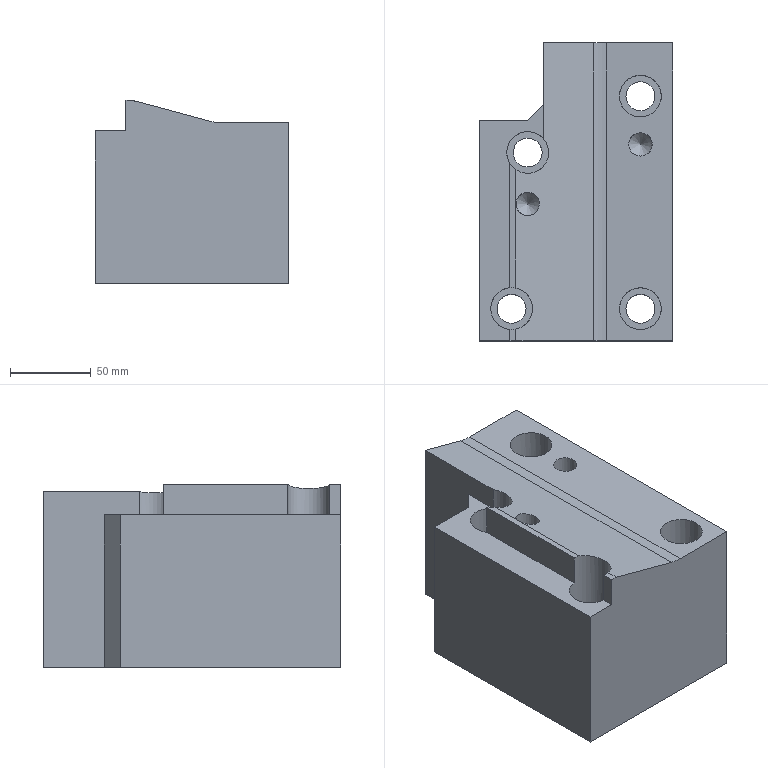Part | STEP file | lll_id4918_x_t | 1 solid | 41 faces | box 120 x 185 x 114 mm | volume 1880331 mm3 | plane 22 | cylinder 15 | cone 2 | torus 2 | commonest cylinder face diameters 18.009 x4 26.008 x4 2 x2 14.506 x2 25 x2 60 x1
STEP:
#1=CARTESIAN_POINT('',(1645.691,-202.,14.));
#2=VERTEX_POINT('',#1);
#3=CARTESIAN_POINT('',(1694.125,-202.,1.022));
#4=VERTEX_POINT('',#3);
#5=CARTESIAN_POINT('',(1684.351,-202.,3.641));
#6=DIRECTION('',(0.9659,0.,-0.2588));
#7=VECTOR('',#6,1.);
#8=LINE('',#5,#7);
#9=EDGE_CURVE('',#2,#4,#8,.T.);
#10=ORIENTED_EDGE('',*,*,#9,.F.);
#11=CARTESIAN_POINT('',(1642.,-202.,14.));
#12=VERTEX_POINT('',#11);
#13=CARTESIAN_POINT('',(1674.,-202.,14.));
#14=DIRECTION('',(1.,0.,0.));
#15=VECTOR('',#14,1.);
#16=LINE('',#13,#15);
#17=EDGE_CURVE('',#12,#2,#16,.T.);
#18=ORIENTED_EDGE('',*,*,#17,.F.);
#19=CARTESIAN_POINT('',(1642.,-202.,-5.));
#20=VERTEX_POINT('',#19);
#21=CARTESIAN_POINT('',(1642.,-202.,-33.25));
#22=DIRECTION('',(0.,0.,-1.));
#23=VECTOR('',#22,1.);
#24=LINE('',#21,#23);
#25=EDGE_CURVE('',#12,#20,#24,.T.);
#26=ORIENTED_EDGE('',*,*,#25,.T.);
#27=CARTESIAN_POINT('',(1623.,-202.,-5.));
#28=VERTEX_POINT('',#27);
#29=CARTESIAN_POINT('',(1674.,-202.,-5.));
#30=DIRECTION('',(1.,0.,0.));
#31=VECTOR('',#30,1.);
#32=LINE('',#29,#31);
#33=EDGE_CURVE('',#28,#20,#32,.T.);
#34=ORIENTED_EDGE('',*,*,#33,.F.);
#35=CARTESIAN_POINT('',(1623.,-202.,-100.));
#36=VERTEX_POINT('',#35);
#37=CARTESIAN_POINT('',(1623.,-202.,-80.));
#38=DIRECTION('',(0.,0.,-1.));
#39=VECTOR('',#38,1.);
#40=LINE('',#37,#39);
#41=EDGE_CURVE('',#28,#36,#40,.T.);
#42=ORIENTED_EDGE('',*,*,#41,.T.);
#43=CARTESIAN_POINT('',(1743.,-202.,-100.));
#44=VERTEX_POINT('',#43);
#45=CARTESIAN_POINT('',(-2196.249,-202.,-100.));
#46=DIRECTION('',(-1.,0.,0.));
#47=VECTOR('',#46,1.);
#48=LINE('',#45,#47);
#49=EDGE_CURVE('',#44,#36,#48,.T.);
#50=ORIENTED_EDGE('',*,*,#49,.F.);
#51=CARTESIAN_POINT('',(1743.,-202.,0.));
#52=VERTEX_POINT('',#51);
#53=CARTESIAN_POINT('',(1743.,-202.,-32.057));
#54=DIRECTION('',(0.,0.,-1.));
#55=VECTOR('',#54,1.);
#56=LINE('',#53,#55);
#57=EDGE_CURVE('',#52,#44,#56,.T.);
#58=ORIENTED_EDGE('',*,*,#57,.F.);
#59=CARTESIAN_POINT('',(1701.89,-202.,0.));
#60=VERTEX_POINT('',#59);
#61=CARTESIAN_POINT('',(12283.883,-202.,0.));
#62=DIRECTION('',(1.,0.,0.));
#63=VECTOR('',#62,1.);
#64=LINE('',#61,#63);
#65=EDGE_CURVE('',#60,#52,#64,.T.);
#66=ORIENTED_EDGE('',*,*,#65,.F.);
#67=CARTESIAN_POINT('',(1701.89,-202.,30.));
#68=DIRECTION('',(0.,1.,0.));
#69=DIRECTION('',(0.,0.,-1.));
#70=AXIS2_PLACEMENT_3D('',#67,#68,#69);
#71=CIRCLE('',#70,30.);
#72=EDGE_CURVE('',#60,#4,#71,.T.);
#73=ORIENTED_EDGE('',*,*,#72,.T.);
#74=EDGE_LOOP('',(#10,#18,#26,#34,#42,#50,#58,#66,#73));
#75=FACE_OUTER_BOUND('',#74,.T.);
#76=CARTESIAN_POINT('',(1674.,-202.,-34.988));
#77=DIRECTION('',(0.,-1.,0.));
#78=DIRECTION('',(0.,0.,-1.));
#79=AXIS2_PLACEMENT_3D('',#76,#77,#78);
#80=PLANE('',#79);
#81=ADVANCED_FACE('',(#75),#80,.T.);
#82=CARTESIAN_POINT('',(1660.253,-117.,10.098));
#83=VERTEX_POINT('',#82);
#84=CARTESIAN_POINT('',(1653.,-117.,12.042));
#85=DIRECTION('',(0.2588,0.,0.9659));
#86=DIRECTION('',(0.9659,0.,-0.2588));
#87=AXIS2_PLACEMENT_3D('',#84,#85,#86);
#88=ELLIPSE('',#87,7.509,7.253);
#89=EDGE_CURVE('',#83,#83,#88,.T.);
#90=ORIENTED_EDGE('',*,*,#89,.F.);
#91=EDGE_LOOP('',(#90));
#92=FACE_BOUND('',#91,.T.);
#93=CARTESIAN_POINT('',(1645.691,-194.722,14.));
#94=VERTEX_POINT('',#93);
#95=CARTESIAN_POINT('',(1645.691,22.5,14.));
#96=DIRECTION('',(0.,-1.,0.));
#97=VECTOR('',#96,1.);
#98=LINE('',#95,#97);
#99=EDGE_CURVE('',#94,#2,#98,.T.);
#100=ORIENTED_EDGE('',*,*,#99,.T.);
#101=ORIENTED_EDGE('',*,*,#9,.T.);
#102=CARTESIAN_POINT('',(1694.125,-17.,1.022));
#103=VERTEX_POINT('',#102);
#104=CARTESIAN_POINT('',(1694.125,13712.786,1.022));
#105=DIRECTION('',(0.,1.,0.));
#106=VECTOR('',#105,1.);
#107=LINE('',#104,#106);
#108=EDGE_CURVE('',#4,#103,#107,.T.);
#109=ORIENTED_EDGE('',*,*,#108,.T.);
#110=CARTESIAN_POINT('',(1663.,-17.,9.362));
#111=VERTEX_POINT('',#110);
#112=CARTESIAN_POINT('',(1667.613,-17.,8.126));
#113=DIRECTION('',(-0.9659,0.,0.2588));
#114=VECTOR('',#113,1.);
#115=LINE('',#112,#114);
#116=EDGE_CURVE('',#103,#111,#115,.T.);
#117=ORIENTED_EDGE('',*,*,#116,.T.);
#118=CARTESIAN_POINT('',(1663.,-76.687,9.362));
#119=VERTEX_POINT('',#118);
#120=CARTESIAN_POINT('',(1663.,-111.,9.362));
#121=DIRECTION('',(0.,-1.,0.));
#122=VECTOR('',#121,1.);
#123=LINE('',#120,#122);
#124=EDGE_CURVE('',#111,#119,#123,.T.);
#125=ORIENTED_EDGE('',*,*,#124,.T.);
#126=CARTESIAN_POINT('',(1645.691,-95.756,14.));
#127=VERTEX_POINT('',#126);
#128=CARTESIAN_POINT('',(1653.,-85.,12.042));
#129=DIRECTION('',(0.2588,0.,0.9659));
#130=DIRECTION('',(0.9659,0.,-0.2588));
#131=AXIS2_PLACEMENT_3D('',#128,#129,#130);
#132=ELLIPSE('',#131,13.463,13.004);
#133=EDGE_CURVE('',#127,#119,#132,.T.);
#134=ORIENTED_EDGE('',*,*,#133,.F.);
#135=CARTESIAN_POINT('',(1645.691,-169.277,14.));
#136=VERTEX_POINT('',#135);
#137=CARTESIAN_POINT('',(1645.691,22.5,14.));
#138=DIRECTION('',(0.,-1.,0.));
#139=VECTOR('',#138,1.);
#140=LINE('',#137,#139);
#141=EDGE_CURVE('',#127,#136,#140,.T.);
#142=ORIENTED_EDGE('',*,*,#141,.T.);
#143=CARTESIAN_POINT('',(1643.,-182.,14.721));
#144=DIRECTION('',(0.2588,0.,0.9659));
#145=DIRECTION('',(0.9659,0.,-0.2588));
#146=AXIS2_PLACEMENT_3D('',#143,#144,#145);
#147=ELLIPSE('',#146,13.463,13.004);
#148=EDGE_CURVE('',#94,#136,#147,.T.);
#149=ORIENTED_EDGE('',*,*,#148,.F.);
#150=EDGE_LOOP('',(#100,#101,#109,#117,#125,#134,#142,#149));
#151=FACE_BOUND('',#150,.T.);
#152=CARTESIAN_POINT('',(1773.773,22.5,-20.319));
#153=DIRECTION('',(-0.2588,0.,-0.9659));
#154=DIRECTION('',(0.9659,0.,-0.2588));
#155=AXIS2_PLACEMENT_3D('',#152,#153,#154);
#156=PLANE('',#155);
#157=ADVANCED_FACE('',(#92,#151),#156,.F.);
#158=CARTESIAN_POINT('',(1639.996,-85.,-50.));
#159=VERTEX_POINT('',#158);
#160=CARTESIAN_POINT('',(1653.,-85.,-50.));
#161=DIRECTION('',(0.,0.,1.));
#162=DIRECTION('',(-1.,0.,0.));
#163=AXIS2_PLACEMENT_3D('',#160,#161,#162);
#164=CIRCLE('',#163,13.004);
#165=EDGE_CURVE('',#159,#159,#164,.T.);
#166=ORIENTED_EDGE('',*,*,#165,.F.);
#167=EDGE_LOOP('',(#166));
#168=FACE_BOUND('',#167,.T.);
#169=CARTESIAN_POINT('',(1642.,-91.936,14.));
#170=VERTEX_POINT('',#169);
#171=CARTESIAN_POINT('',(1653.,-85.,14.));
#172=DIRECTION('',(0.,0.,-1.));
#173=DIRECTION('',(1.,0.,0.));
#174=AXIS2_PLACEMENT_3D('',#171,#172,#173);
#175=CIRCLE('',#174,13.004);
#176=EDGE_CURVE('',#127,#170,#175,.T.);
#177=ORIENTED_EDGE('',*,*,#176,.F.);
#178=ORIENTED_EDGE('',*,*,#133,.T.);
#179=CARTESIAN_POINT('',(1663.,-76.687,-5.));
#180=VERTEX_POINT('',#179);
#181=CARTESIAN_POINT('',(1663.,-76.687,3.53));
#182=DIRECTION('',(0.,0.,1.));
#183=VECTOR('',#182,1.);
#184=LINE('',#181,#183);
#185=EDGE_CURVE('',#180,#119,#184,.T.);
#186=ORIENTED_EDGE('',*,*,#185,.F.);
#187=CARTESIAN_POINT('',(1642.,-91.936,-5.));
#188=VERTEX_POINT('',#187);
#189=CARTESIAN_POINT('',(1653.,-85.,-5.));
#190=DIRECTION('',(0.,0.,-1.));
#191=DIRECTION('',(1.,0.,0.));
#192=AXIS2_PLACEMENT_3D('',#189,#190,#191);
#193=CIRCLE('',#192,13.004);
#194=EDGE_CURVE('',#188,#180,#193,.T.);
#195=ORIENTED_EDGE('',*,*,#194,.F.);
#196=CARTESIAN_POINT('',(1642.,-91.936,13.5));
#197=DIRECTION('',(0.,0.,-1.));
#198=VECTOR('',#197,1.);
#199=LINE('',#196,#198);
#200=EDGE_CURVE('',#170,#188,#199,.T.);
#201=ORIENTED_EDGE('',*,*,#200,.F.);
#202=EDGE_LOOP('',(#177,#178,#186,#195,#201));
#203=FACE_BOUND('',#202,.T.);
#204=CARTESIAN_POINT('',(1653.,-85.,13.5));
#205=DIRECTION('',(0.,0.,-1.));
#206=DIRECTION('',(-1.,0.,0.));
#207=AXIS2_PLACEMENT_3D('',#204,#205,#206);
#208=CYLINDRICAL_SURFACE('',#207,13.004);
#209=ADVANCED_FACE('',(#168,#203),#208,.F.);
#210=CARTESIAN_POINT('',(1629.996,-182.,-50.));
#211=VERTEX_POINT('',#210);
#212=CARTESIAN_POINT('',(1643.,-182.,-50.));
#213=DIRECTION('',(0.,0.,1.));
#214=DIRECTION('',(-1.,0.,0.));
#215=AXIS2_PLACEMENT_3D('',#212,#213,#214);
#216=CIRCLE('',#215,13.004);
#217=EDGE_CURVE('',#211,#211,#216,.T.);
#218=ORIENTED_EDGE('',*,*,#217,.F.);
#219=EDGE_LOOP('',(#218));
#220=FACE_BOUND('',#219,.T.);
#221=CARTESIAN_POINT('',(1642.,-194.965,14.));
#222=VERTEX_POINT('',#221);
#223=CARTESIAN_POINT('',(1643.,-182.,14.));
#224=DIRECTION('',(0.,0.,-1.));
#225=DIRECTION('',(1.,0.,0.));
#226=AXIS2_PLACEMENT_3D('',#223,#224,#225);
#227=CIRCLE('',#226,13.004);
#228=EDGE_CURVE('',#94,#222,#227,.T.);
#229=ORIENTED_EDGE('',*,*,#228,.F.);
#230=ORIENTED_EDGE('',*,*,#148,.T.);
#231=CARTESIAN_POINT('',(1642.,-169.034,14.));
#232=VERTEX_POINT('',#231);
#233=CARTESIAN_POINT('',(1643.,-182.,14.));
#234=DIRECTION('',(0.,0.,-1.));
#235=DIRECTION('',(1.,0.,0.));
#236=AXIS2_PLACEMENT_3D('',#233,#234,#235);
#237=CIRCLE('',#236,13.004);
#238=EDGE_CURVE('',#232,#136,#237,.T.);
#239=ORIENTED_EDGE('',*,*,#238,.F.);
#240=CARTESIAN_POINT('',(1642.,-169.034,-5.));
#241=VERTEX_POINT('',#240);
#242=CARTESIAN_POINT('',(1642.,-169.034,13.5));
#243=DIRECTION('',(0.,0.,-1.));
#244=VECTOR('',#243,1.);
#245=LINE('',#242,#244);
#246=EDGE_CURVE('',#232,#241,#245,.T.);
#247=ORIENTED_EDGE('',*,*,#246,.T.);
#248=CARTESIAN_POINT('',(1642.,-194.965,-5.));
#249=VERTEX_POINT('',#248);
#250=CARTESIAN_POINT('',(1643.,-182.,-5.));
#251=DIRECTION('',(0.,0.,1.));
#252=DIRECTION('',(1.,0.,0.));
#253=AXIS2_PLACEMENT_3D('',#250,#251,#252);
#254=CIRCLE('',#253,13.004);
#255=EDGE_CURVE('',#241,#249,#254,.T.);
#256=ORIENTED_EDGE('',*,*,#255,.T.);
#257=CARTESIAN_POINT('',(1642.,-194.965,13.5));
#258=DIRECTION('',(0.,0.,1.));
#259=VECTOR('',#258,1.);
#260=LINE('',#257,#259);
#261=EDGE_CURVE('',#249,#222,#260,.T.);
#262=ORIENTED_EDGE('',*,*,#261,.T.);
#263=EDGE_LOOP('',(#229,#230,#239,#247,#256,#262));
#264=FACE_BOUND('',#263,.T.);
#265=CARTESIAN_POINT('',(1643.,-182.,13.5));
#266=DIRECTION('',(0.,0.,-1.));
#267=DIRECTION('',(-1.,0.,0.));
#268=AXIS2_PLACEMENT_3D('',#265,#266,#267);
#269=CYLINDRICAL_SURFACE('',#268,13.004);
#270=ADVANCED_FACE('',(#220,#264),#269,.F.);
#271=ORIENTED_EDGE('',*,*,#25,.F.);
#272=CARTESIAN_POINT('',(1642.,-111.,14.));
#273=DIRECTION('',(0.,1.,0.));
#274=VECTOR('',#273,1.);
#275=LINE('',#272,#274);
#276=EDGE_CURVE('',#12,#222,#275,.T.);
#277=ORIENTED_EDGE('',*,*,#276,.T.);
#278=ORIENTED_EDGE('',*,*,#261,.F.);
#279=CARTESIAN_POINT('',(1642.,-111.,-5.));
#280=DIRECTION('',(0.,1.,0.));
#281=VECTOR('',#280,1.);
#282=LINE('',#279,#281);
#283=EDGE_CURVE('',#20,#249,#282,.T.);
#284=ORIENTED_EDGE('',*,*,#283,.F.);
#285=EDGE_LOOP('',(#271,#277,#278,#284));
#286=FACE_OUTER_BOUND('',#285,.T.);
#287=CARTESIAN_POINT('',(1642.,-111.,-33.25));
#288=DIRECTION('',(-1.,0.,0.));
#289=DIRECTION('',(0.,0.,-1.));
#290=AXIS2_PLACEMENT_3D('',#287,#288,#289);
#291=PLANE('',#290);
#292=ADVANCED_FACE('',(#286),#291,.T.);
#293=ORIENTED_EDGE('',*,*,#246,.F.);
#294=CARTESIAN_POINT('',(1642.,-111.,14.));
#295=DIRECTION('',(0.,1.,0.));
#296=VECTOR('',#295,1.);
#297=LINE('',#294,#296);
#298=EDGE_CURVE('',#232,#170,#297,.T.);
#299=ORIENTED_EDGE('',*,*,#298,.T.);
#300=ORIENTED_EDGE('',*,*,#200,.T.);
#301=CARTESIAN_POINT('',(1642.,-111.,-5.));
#302=DIRECTION('',(0.,1.,0.));
#303=VECTOR('',#302,1.);
#304=LINE('',#301,#303);
#305=EDGE_CURVE('',#241,#188,#304,.T.);
#306=ORIENTED_EDGE('',*,*,#305,.F.);
#307=EDGE_LOOP('',(#293,#299,#300,#306));
#308=FACE_OUTER_BOUND('',#307,.T.);
#309=CARTESIAN_POINT('',(1642.,-111.,-33.25));
#310=DIRECTION('',(-1.,0.,0.));
#311=DIRECTION('',(0.,0.,-1.));
#312=AXIS2_PLACEMENT_3D('',#309,#310,#311);
#313=PLANE('',#312);
#314=ADVANCED_FACE('',(#308),#313,.T.);
#315=CARTESIAN_POINT('',(1663.,-55.,-5.));
#316=VERTEX_POINT('',#315);
#317=CARTESIAN_POINT('',(1663.,-111.,-5.));
#318=DIRECTION('',(0.,1.,0.));
#319=VECTOR('',#318,1.);
#320=LINE('',#317,#319);
#321=EDGE_CURVE('',#180,#316,#320,.T.);
#322=ORIENTED_EDGE('',*,*,#321,.F.);
#323=ORIENTED_EDGE('',*,*,#185,.T.);
#324=ORIENTED_EDGE('',*,*,#124,.F.);
#325=CARTESIAN_POINT('',(1663.,-17.,-100.));
#326=VERTEX_POINT('',#325);
#327=CARTESIAN_POINT('',(1663.,-17.,-42.5));
#328=DIRECTION('',(0.,0.,1.));
#329=VECTOR('',#328,1.);
#330=LINE('',#327,#329);
#331=EDGE_CURVE('',#326,#111,#330,.T.);
#332=ORIENTED_EDGE('',*,*,#331,.F.);
#333=CARTESIAN_POINT('',(1663.,-55.,-100.));
#334=VERTEX_POINT('',#333);
#335=CARTESIAN_POINT('',(1663.,-1.,-100.));
#336=DIRECTION('',(0.,1.,0.));
#337=VECTOR('',#336,1.);
#338=LINE('',#335,#337);
#339=EDGE_CURVE('',#334,#326,#338,.T.);
#340=ORIENTED_EDGE('',*,*,#339,.F.);
#341=CARTESIAN_POINT('',(1663.,-55.,-80.));
#342=DIRECTION('',(0.,0.,-1.));
#343=VECTOR('',#342,1.);
#344=LINE('',#341,#343);
#345=EDGE_CURVE('',#316,#334,#344,.T.);
#346=ORIENTED_EDGE('',*,*,#345,.F.);
#347=EDGE_LOOP('',(#322,#323,#324,#332,#340,#346));
#348=FACE_OUTER_BOUND('',#347,.T.);
#349=CARTESIAN_POINT('',(1663.,-111.,-42.5));
#350=DIRECTION('',(-1.,0.,0.));
#351=DIRECTION('',(0.,0.,-1.));
#352=AXIS2_PLACEMENT_3D('',#349,#350,#351);
#353=PLANE('',#352);
#354=ADVANCED_FACE('',(#348),#353,.T.);
#355=ORIENTED_EDGE('',*,*,#116,.F.);
#356=CARTESIAN_POINT('',(1701.89,-17.,0.));
#357=VERTEX_POINT('',#356);
#358=CARTESIAN_POINT('',(1701.89,-17.,30.));
#359=DIRECTION('',(0.,1.,0.));
#360=DIRECTION('',(0.,0.,1.));
#361=AXIS2_PLACEMENT_3D('',#358,#359,#360);
#362=CIRCLE('',#361,30.);
#363=EDGE_CURVE('',#357,#103,#362,.T.);
#364=ORIENTED_EDGE('',*,*,#363,.F.);
#365=CARTESIAN_POINT('',(1743.,-17.,0.));
#366=VERTEX_POINT('',#365);
#367=CARTESIAN_POINT('',(12283.883,-17.,0.));
#368=DIRECTION('',(-1.,0.,0.));
#369=VECTOR('',#368,1.);
#370=LINE('',#367,#369);
#371=EDGE_CURVE('',#366,#357,#370,.T.);
#372=ORIENTED_EDGE('',*,*,#371,.F.);
#373=CARTESIAN_POINT('',(1743.,-17.,-100.));
#374=VERTEX_POINT('',#373);
#375=CARTESIAN_POINT('',(1743.,-17.,-80.));
#376=DIRECTION('',(0.,0.,-1.));
#377=VECTOR('',#376,1.);
#378=LINE('',#375,#377);
#379=EDGE_CURVE('',#366,#374,#378,.T.);
#380=ORIENTED_EDGE('',*,*,#379,.T.);
#381=CARTESIAN_POINT('',(-2196.249,-17.,-100.));
#382=DIRECTION('',(1.,0.,0.));
#383=VECTOR('',#382,1.);
#384=LINE('',#381,#383);
#385=EDGE_CURVE('',#326,#374,#384,.T.);
#386=ORIENTED_EDGE('',*,*,#385,.F.);
#387=ORIENTED_EDGE('',*,*,#331,.T.);
#388=EDGE_LOOP('',(#355,#364,#372,#380,#386,#387));
#389=FACE_OUTER_BOUND('',#388,.T.);
#390=CARTESIAN_POINT('',(1644.,-17.,-80.));
#391=DIRECTION('',(0.,1.,0.));
#392=DIRECTION('',(0.,0.,1.));
#393=AXIS2_PLACEMENT_3D('',#390,#391,#392);
#394=PLANE('',#393);
#395=ADVANCED_FACE('',(#389),#394,.T.);
#396=CARTESIAN_POINT('',(1660.,-147.,-100.));
#397=VERTEX_POINT('',#396);
#398=CARTESIAN_POINT('',(1660.,-122.,-100.));
#399=VERTEX_POINT('',#398);
#400=CARTESIAN_POINT('',(1660.,-134.5,-100.));
#401=DIRECTION('',(0.,0.,-1.));
#402=DIRECTION('',(-1.,0.,0.));
#403=AXIS2_PLACEMENT_3D('',#400,#401,#402);
#404=CIRCLE('',#403,12.5);
#405=EDGE_CURVE('',#397,#399,#404,.T.);
#406=ORIENTED_EDGE('',*,*,#405,.F.);
#407=CARTESIAN_POINT('',(1716.,-147.,-100.));
#408=VERTEX_POINT('',#407);
#409=CARTESIAN_POINT('',(-2196.249,-147.,-100.));
#410=DIRECTION('',(-1.,0.,0.));
#411=VECTOR('',#410,1.);
#412=LINE('',#409,#411);
#413=EDGE_CURVE('',#408,#397,#412,.T.);
#414=ORIENTED_EDGE('',*,*,#413,.F.);
#415=CARTESIAN_POINT('',(1716.,-122.,-100.));
#416=VERTEX_POINT('',#415);
#417=CARTESIAN_POINT('',(1716.,-134.5,-100.));
#418=DIRECTION('',(0.,0.,-1.));
#419=DIRECTION('',(-1.,0.,0.));
#420=AXIS2_PLACEMENT_3D('',#417,#418,#419);
#421=CIRCLE('',#420,12.5);
#422=EDGE_CURVE('',#416,#408,#421,.T.);
#423=ORIENTED_EDGE('',*,*,#422,.F.);
#424=CARTESIAN_POINT('',(-2196.249,-122.,-100.));
#425=DIRECTION('',(1.,0.,0.));
#426=VECTOR('',#425,1.);
#427=LINE('',#424,#426);
#428=EDGE_CURVE('',#399,#416,#427,.T.);
#429=ORIENTED_EDGE('',*,*,#428,.F.);
#430=EDGE_LOOP('',(#406,#414,#423,#429));
#431=FACE_BOUND('',#430,.T.);
#432=CARTESIAN_POINT('',(1713.995,-182.,-100.));
#433=VERTEX_POINT('',#432);
#434=CARTESIAN_POINT('',(1723.,-182.,-100.));
#435=DIRECTION('',(0.,0.,1.));
#436=DIRECTION('',(-1.,0.,0.));
#437=AXIS2_PLACEMENT_3D('',#434,#435,#436);
#438=CIRCLE('',#437,9.005);
#439=EDGE_CURVE('',#433,#433,#438,.T.);
#440=ORIENTED_EDGE('',*,*,#439,.T.);
#441=EDGE_LOOP('',(#440));
#442=FACE_BOUND('',#441,.T.);
#443=CARTESIAN_POINT('',(1713.995,-50.,-100.));
#444=VERTEX_POINT('',#443);
#445=CARTESIAN_POINT('',(1723.,-50.,-100.));
#446=DIRECTION('',(0.,0.,1.));
#447=DIRECTION('',(-1.,0.,0.));
#448=AXIS2_PLACEMENT_3D('',#445,#446,#447);
#449=CIRCLE('',#448,9.005);
#450=EDGE_CURVE('',#444,#444,#449,.T.);
#451=ORIENTED_EDGE('',*,*,#450,.T.);
#452=EDGE_LOOP('',(#451));
#453=FACE_BOUND('',#452,.T.);
#454=ORIENTED_EDGE('',*,*,#385,.T.);
#455=CARTESIAN_POINT('',(1743.,-1.,-100.));
#456=DIRECTION('',(0.,1.,0.));
#457=VECTOR('',#456,1.);
#458=LINE('',#455,#457);
#459=EDGE_CURVE('',#44,#374,#458,.T.);
#460=ORIENTED_EDGE('',*,*,#459,.F.);
#461=ORIENTED_EDGE('',*,*,#49,.T.);
#462=CARTESIAN_POINT('',(1623.,-65.,-100.));
#463=VERTEX_POINT('',#462);
#464=CARTESIAN_POINT('',(1623.,-1.,-100.));
#465=DIRECTION('',(0.,1.,0.));
#466=VECTOR('',#465,1.);
#467=LINE('',#464,#466);
#468=EDGE_CURVE('',#36,#463,#467,.T.);
#469=ORIENTED_EDGE('',*,*,#468,.T.);
#470=CARTESIAN_POINT('',(1653.,-65.,-100.));
#471=VERTEX_POINT('',#470);
#472=CARTESIAN_POINT('',(-2196.249,-65.,-100.));
#473=DIRECTION('',(1.,0.,0.));
#474=VECTOR('',#473,1.);
#475=LINE('',#472,#474);
#476=EDGE_CURVE('',#463,#471,#475,.T.);
#477=ORIENTED_EDGE('',*,*,#476,.T.);
#478=CARTESIAN_POINT('',(-239.625,-1957.625,-100.));
#479=DIRECTION('',(-0.7071,-0.7071,0.));
#480=VECTOR('',#479,1.);
#481=LINE('',#478,#480);
#482=EDGE_CURVE('',#334,#471,#481,.T.);
#483=ORIENTED_EDGE('',*,*,#482,.F.);
#484=ORIENTED_EDGE('',*,*,#339,.T.);
#485=EDGE_LOOP('',(#454,#460,#461,#469,#477,#483,#484));
#486=FACE_BOUND('',#485,.T.);
#487=CARTESIAN_POINT('',(1643.995,-85.,-100.));
#488=VERTEX_POINT('',#487);
#489=CARTESIAN_POINT('',(1653.,-85.,-100.));
#490=DIRECTION('',(0.,0.,1.));
#491=DIRECTION('',(-1.,0.,0.));
#492=AXIS2_PLACEMENT_3D('',#489,#490,#491);
#493=CIRCLE('',#492,9.005);
#494=EDGE_CURVE('',#488,#488,#493,.T.);
#495=ORIENTED_EDGE('',*,*,#494,.T.);
#496=EDGE_LOOP('',(#495));
#497=FACE_BOUND('',#496,.T.);
#498=CARTESIAN_POINT('',(1633.995,-182.,-100.));
#499=VERTEX_POINT('',#498);
#500=CARTESIAN_POINT('',(1643.,-182.,-100.));
#501=DIRECTION('',(0.,0.,1.));
#502=DIRECTION('',(-1.,0.,0.));
#503=AXIS2_PLACEMENT_3D('',#500,#501,#502);
#504=CIRCLE('',#503,9.005);
#505=EDGE_CURVE('',#499,#499,#504,.T.);
#506=ORIENTED_EDGE('',*,*,#505,.T.);
#507=EDGE_LOOP('',(#506));
#508=FACE_BOUND('',#507,.T.);
#509=CARTESIAN_POINT('',(-2196.249,-1.,-100.));
#510=DIRECTION('',(0.,0.,-1.));
#511=DIRECTION('',(1.,0.,0.));
#512=AXIS2_PLACEMENT_3D('',#509,#510,#511);
#513=PLANE('',#512);
#514=ADVANCED_FACE('',(#431,#442,#453,#486,#497,#508),#513,.T.);
#515=ORIENTED_EDGE('',*,*,#165,.T.);
#516=EDGE_LOOP('',(#515));
#517=FACE_BOUND('',#516,.T.);
#518=CARTESIAN_POINT('',(1662.005,-85.,-50.));
#519=VERTEX_POINT('',#518);
#520=CARTESIAN_POINT('',(1653.,-85.,-50.));
#521=DIRECTION('',(0.,0.,1.));
#522=DIRECTION('',(1.,0.,0.));
#523=AXIS2_PLACEMENT_3D('',#520,#521,#522);
#524=CIRCLE('',#523,9.005);
#525=EDGE_CURVE('',#519,#519,#524,.T.);
#526=ORIENTED_EDGE('',*,*,#525,.F.);
#527=EDGE_LOOP('',(#526));
#528=FACE_BOUND('',#527,.T.);
#529=CARTESIAN_POINT('',(1653.,-85.,-50.));
#530=DIRECTION('',(0.,0.,-1.));
#531=DIRECTION('',(1.,0.,0.));
#532=AXIS2_PLACEMENT_3D('',#529,#530,#531);
#533=PLANE('',#532);
#534=ADVANCED_FACE('',(#517,#528),#533,.F.);
#535=ORIENTED_EDGE('',*,*,#57,.T.);
#536=ORIENTED_EDGE('',*,*,#459,.T.);
#537=ORIENTED_EDGE('',*,*,#379,.F.);
#538=CARTESIAN_POINT('',(1743.,13712.786,0.));
#539=DIRECTION('',(0.,-1.,0.));
#540=VECTOR('',#539,1.);
#541=LINE('',#538,#540);
#542=EDGE_CURVE('',#366,#52,#541,.T.);
#543=ORIENTED_EDGE('',*,*,#542,.T.);
#544=EDGE_LOOP('',(#535,#536,#537,#543));
#545=FACE_OUTER_BOUND('',#544,.T.);
#546=CARTESIAN_POINT('',(1743.,-187.,-32.057));
#547=DIRECTION('',(-1.,0.,0.));
#548=DIRECTION('',(0.,0.,-1.));
#549=AXIS2_PLACEMENT_3D('',#546,#547,#548);
#550=PLANE('',#549);
#551=ADVANCED_FACE('',(#545),#550,.F.);
#552=CARTESIAN_POINT('',(1723.,-72.747,0.));
#553=VERTEX_POINT('',#552);
#554=CARTESIAN_POINT('',(1723.,-80.,0.));
#555=DIRECTION('',(0.,0.,1.));
#556=DIRECTION('',(0.,1.,0.));
#557=AXIS2_PLACEMENT_3D('',#554,#555,#556);
#558=CIRCLE('',#557,7.253);
#559=EDGE_CURVE('',#553,#553,#558,.T.);
#560=ORIENTED_EDGE('',*,*,#559,.F.);
#561=EDGE_LOOP('',(#560));
#562=FACE_BOUND('',#561,.T.);
#563=CARTESIAN_POINT('',(1723.,-168.996,0.));
#564=VERTEX_POINT('',#563);
#565=CARTESIAN_POINT('',(1723.,-182.,0.));
#566=DIRECTION('',(0.,0.,1.));
#567=DIRECTION('',(0.,1.,0.));
#568=AXIS2_PLACEMENT_3D('',#565,#566,#567);
#569=CIRCLE('',#568,13.004);
#570=EDGE_CURVE('',#564,#564,#569,.T.);
#571=ORIENTED_EDGE('',*,*,#570,.F.);
#572=EDGE_LOOP('',(#571));
#573=FACE_BOUND('',#572,.T.);
#574=CARTESIAN_POINT('',(1723.,-36.996,0.));
#575=VERTEX_POINT('',#574);
#576=CARTESIAN_POINT('',(1723.,-50.,0.));
#577=DIRECTION('',(0.,0.,1.));
#578=DIRECTION('',(0.,1.,0.));
#579=AXIS2_PLACEMENT_3D('',#576,#577,#578);
#580=CIRCLE('',#579,13.004);
#581=EDGE_CURVE('',#575,#575,#580,.T.);
#582=ORIENTED_EDGE('',*,*,#581,.F.);
#583=EDGE_LOOP('',(#582));
#584=FACE_BOUND('',#583,.T.);
#585=ORIENTED_EDGE('',*,*,#65,.T.);
#586=ORIENTED_EDGE('',*,*,#542,.F.);
#587=ORIENTED_EDGE('',*,*,#371,.T.);
#588=CARTESIAN_POINT('',(1701.89,13712.786,0.));
#589=DIRECTION('',(0.,1.,0.));
#590=VECTOR('',#589,1.);
#591=LINE('',#588,#590);
#592=EDGE_CURVE('',#60,#357,#591,.T.);
#593=ORIENTED_EDGE('',*,*,#592,.F.);
#594=EDGE_LOOP('',(#585,#586,#587,#593));
#595=FACE_BOUND('',#594,.T.);
#596=CARTESIAN_POINT('',(12283.883,13712.786,0.));
#597=DIRECTION('',(0.,0.,-1.));
#598=DIRECTION('',(1.,0.,0.));
#599=AXIS2_PLACEMENT_3D('',#596,#597,#598);
#600=PLANE('',#599);
#601=ADVANCED_FACE('',(#562,#573,#584,#595),#600,.F.);
#602=ORIENTED_EDGE('',*,*,#72,.F.);
#603=ORIENTED_EDGE('',*,*,#592,.T.);
#604=ORIENTED_EDGE('',*,*,#363,.T.);
#605=ORIENTED_EDGE('',*,*,#108,.F.);
#606=EDGE_LOOP('',(#602,#603,#604,#605));
#607=FACE_OUTER_BOUND('',#606,.T.);
#608=CARTESIAN_POINT('',(1701.89,13712.786,30.));
#609=DIRECTION('',(0.,1.,0.));
#610=DIRECTION('',(1.,0.,0.));
#611=AXIS2_PLACEMENT_3D('',#608,#609,#610);
#612=CYLINDRICAL_SURFACE('',#611,30.);
#613=ADVANCED_FACE('',(#607),#612,.F.);
#614=CARTESIAN_POINT('',(1709.996,-50.,-50.));
#615=VERTEX_POINT('',#614);
#616=CARTESIAN_POINT('',(1723.,-50.,-50.));
#617=DIRECTION('',(0.,0.,1.));
#618=DIRECTION('',(-1.,0.,0.));
#619=AXIS2_PLACEMENT_3D('',#616,#617,#618);
#620=CIRCLE('',#619,13.004);
#621=EDGE_CURVE('',#615,#615,#620,.T.);
#622=ORIENTED_EDGE('',*,*,#621,.F.);
#623=EDGE_LOOP('',(#622));
#624=FACE_BOUND('',#623,.T.);
#625=ORIENTED_EDGE('',*,*,#581,.T.);
#626=EDGE_LOOP('',(#625));
#627=FACE_BOUND('',#626,.T.);
#628=CARTESIAN_POINT('',(1723.,-50.,13.5));
#629=DIRECTION('',(0.,0.,-1.));
#630=DIRECTION('',(-1.,0.,0.));
#631=AXIS2_PLACEMENT_3D('',#628,#629,#630);
#632=CYLINDRICAL_SURFACE('',#631,13.004);
#633=ADVANCED_FACE('',(#624,#627),#632,.F.);
#634=ORIENTED_EDGE('',*,*,#450,.F.);
#635=EDGE_LOOP('',(#634));
#636=FACE_BOUND('',#635,.T.);
#637=CARTESIAN_POINT('',(1732.005,-50.,-50.));
#638=VERTEX_POINT('',#637);
#639=CARTESIAN_POINT('',(1723.,-50.,-50.));
#640=DIRECTION('',(0.,0.,1.));
#641=DIRECTION('',(1.,0.,0.));
#642=AXIS2_PLACEMENT_3D('',#639,#640,#641);
#643=CIRCLE('',#642,9.005);
#644=EDGE_CURVE('',#638,#638,#643,.T.);
#645=ORIENTED_EDGE('',*,*,#644,.T.);
#646=EDGE_LOOP('',(#645));
#647=FACE_BOUND('',#646,.T.);
#648=CARTESIAN_POINT('',(1723.,-50.,15.5));
#649=DIRECTION('',(0.,0.,-1.));
#650=DIRECTION('',(-1.,0.,0.));
#651=AXIS2_PLACEMENT_3D('',#648,#649,#650);
#652=CYLINDRICAL_SURFACE('',#651,9.005);
#653=ADVANCED_FACE('',(#636,#647),#652,.F.);
#654=ORIENTED_EDGE('',*,*,#644,.F.);
#655=EDGE_LOOP('',(#654));
#656=FACE_BOUND('',#655,.T.);
#657=ORIENTED_EDGE('',*,*,#621,.T.);
#658=EDGE_LOOP('',(#657));
#659=FACE_BOUND('',#658,.T.);
#660=CARTESIAN_POINT('',(1723.,-40.,-50.));
#661=DIRECTION('',(0.,0.,-1.));
#662=DIRECTION('',(1.,0.,0.));
#663=AXIS2_PLACEMENT_3D('',#660,#661,#662);
#664=PLANE('',#663);
#665=ADVANCED_FACE('',(#656,#659),#664,.F.);
#666=CARTESIAN_POINT('',(1736.004,-182.,-50.));
#667=VERTEX_POINT('',#666);
#668=CARTESIAN_POINT('',(1723.,-182.,-50.));
#669=DIRECTION('',(0.,0.,1.));
#670=DIRECTION('',(1.,0.,0.));
#671=AXIS2_PLACEMENT_3D('',#668,#669,#670);
#672=CIRCLE('',#671,13.004);
#673=EDGE_CURVE('',#667,#667,#672,.T.);
#674=ORIENTED_EDGE('',*,*,#673,.F.);
#675=EDGE_LOOP('',(#674));
#676=FACE_BOUND('',#675,.T.);
#677=ORIENTED_EDGE('',*,*,#570,.T.);
#678=EDGE_LOOP('',(#677));
#679=FACE_BOUND('',#678,.T.);
#680=CARTESIAN_POINT('',(1723.,-182.,13.5));
#681=DIRECTION('',(0.,0.,-1.));
#682=DIRECTION('',(-1.,0.,0.));
#683=AXIS2_PLACEMENT_3D('',#680,#681,#682);
#684=CYLINDRICAL_SURFACE('',#683,13.004);
#685=ADVANCED_FACE('',(#676,#679),#684,.F.);
#686=ORIENTED_EDGE('',*,*,#439,.F.);
#687=EDGE_LOOP('',(#686));
#688=FACE_BOUND('',#687,.T.);
#689=CARTESIAN_POINT('',(1732.005,-182.,-50.));
#690=VERTEX_POINT('',#689);
#691=CARTESIAN_POINT('',(1723.,-182.,-50.));
#692=DIRECTION('',(0.,0.,1.));
#693=DIRECTION('',(1.,0.,0.));
#694=AXIS2_PLACEMENT_3D('',#691,#692,#693);
#695=CIRCLE('',#694,9.005);
#696=EDGE_CURVE('',#690,#690,#695,.T.);
#697=ORIENTED_EDGE('',*,*,#696,.T.);
#698=EDGE_LOOP('',(#697));
#699=FACE_BOUND('',#698,.T.);
#700=CARTESIAN_POINT('',(1723.,-182.,15.5));
#701=DIRECTION('',(0.,0.,-1.));
#702=DIRECTION('',(-1.,0.,0.));
#703=AXIS2_PLACEMENT_3D('',#700,#701,#702);
#704=CYLINDRICAL_SURFACE('',#703,9.005);
#705=ADVANCED_FACE('',(#688,#699),#704,.F.);
#706=ORIENTED_EDGE('',*,*,#696,.F.);
#707=EDGE_LOOP('',(#706));
#708=FACE_BOUND('',#707,.T.);
#709=ORIENTED_EDGE('',*,*,#673,.T.);
#710=EDGE_LOOP('',(#709));
#711=FACE_BOUND('',#710,.T.);
#712=CARTESIAN_POINT('',(1723.,-182.,-50.));
#713=DIRECTION('',(0.,0.,-1.));
#714=DIRECTION('',(1.,0.,0.));
#715=AXIS2_PLACEMENT_3D('',#712,#713,#714);
#716=PLANE('',#715);
#717=ADVANCED_FACE('',(#708,#711),#716,.F.);
#718=CARTESIAN_POINT('',(1730.253,-80.,-22.253));
#719=VERTEX_POINT('',#718);
#720=CARTESIAN_POINT('',(1723.,-80.,-22.253));
#721=DIRECTION('',(0.,0.,1.));
#722=DIRECTION('',(1.,0.,0.));
#723=AXIS2_PLACEMENT_3D('',#720,#721,#722);
#724=CIRCLE('',#723,7.253);
#725=EDGE_CURVE('',#719,#719,#724,.T.);
#726=ORIENTED_EDGE('',*,*,#725,.F.);
#727=EDGE_LOOP('',(#726));
#728=FACE_BOUND('',#727,.T.);
#729=ORIENTED_EDGE('',*,*,#559,.T.);
#730=EDGE_LOOP('',(#729));
#731=FACE_BOUND('',#730,.T.);
#732=CARTESIAN_POINT('',(1723.,-80.,15.5));
#733=DIRECTION('',(0.,0.,-1.));
#734=DIRECTION('',(-1.,0.,0.));
#735=AXIS2_PLACEMENT_3D('',#732,#733,#734);
#736=CYLINDRICAL_SURFACE('',#735,7.253);
#737=ADVANCED_FACE('',(#728,#731),#736,.F.);
#738=CARTESIAN_POINT('',(1723.,-80.,-29.506));
#739=VERTEX_POINT('',#738);
#740=VERTEX_LOOP('',#739);
#741=FACE_BOUND('',#740,.T.);
#742=ORIENTED_EDGE('',*,*,#725,.T.);
#743=EDGE_LOOP('',(#742));
#744=FACE_BOUND('',#743,.T.);
#745=CARTESIAN_POINT('',(1723.,-80.,-22.253));
#746=DIRECTION('',(0.,0.,1.));
#747=DIRECTION('',(-1.,0.,0.));
#748=AXIS2_PLACEMENT_3D('',#745,#746,#747);
#749=CONICAL_SURFACE('',#748,7.253,45.);
#750=ADVANCED_FACE('',(#741,#744),#749,.F.);
#751=CARTESIAN_POINT('',(1653.,-117.,-29.506));
#752=VERTEX_POINT('',#751);
#753=VERTEX_LOOP('',#752);
#754=FACE_BOUND('',#753,.T.);
#755=CARTESIAN_POINT('',(1660.253,-117.,-22.253));
#756=VERTEX_POINT('',#755);
#757=CARTESIAN_POINT('',(1653.,-117.,-22.253));
#758=DIRECTION('',(0.,0.,-1.));
#759=DIRECTION('',(1.,0.,0.));
#760=AXIS2_PLACEMENT_3D('',#757,#758,#759);
#761=CIRCLE('',#760,7.253);
#762=EDGE_CURVE('',#756,#756,#761,.T.);
#763=ORIENTED_EDGE('',*,*,#762,.F.);
#764=EDGE_LOOP('',(#763));
#765=FACE_BOUND('',#764,.T.);
#766=CARTESIAN_POINT('',(1653.,-117.,-22.253));
#767=DIRECTION('',(0.,0.,1.));
#768=DIRECTION('',(-1.,0.,0.));
#769=AXIS2_PLACEMENT_3D('',#766,#767,#768);
#770=CONICAL_SURFACE('',#769,7.253,45.);
#771=ADVANCED_FACE('',(#754,#765),#770,.F.);
#772=ORIENTED_EDGE('',*,*,#217,.T.);
#773=EDGE_LOOP('',(#772));
#774=FACE_BOUND('',#773,.T.);
#775=CARTESIAN_POINT('',(1652.005,-182.,-50.));
#776=VERTEX_POINT('',#775);
#777=CARTESIAN_POINT('',(1643.,-182.,-50.));
#778=DIRECTION('',(0.,0.,1.));
#779=DIRECTION('',(1.,0.,0.));
#780=AXIS2_PLACEMENT_3D('',#777,#778,#779);
#781=CIRCLE('',#780,9.005);
#782=EDGE_CURVE('',#776,#776,#781,.T.);
#783=ORIENTED_EDGE('',*,*,#782,.F.);
#784=EDGE_LOOP('',(#783));
#785=FACE_BOUND('',#784,.T.);
#786=CARTESIAN_POINT('',(1643.,-182.,-50.));
#787=DIRECTION('',(0.,0.,-1.));
#788=DIRECTION('',(1.,0.,0.));
#789=AXIS2_PLACEMENT_3D('',#786,#787,#788);
#790=PLANE('',#789);
#791=ADVANCED_FACE('',(#774,#785),#790,.F.);
#792=ORIENTED_EDGE('',*,*,#762,.T.);
#793=EDGE_LOOP('',(#792));
#794=FACE_BOUND('',#793,.T.);
#795=ORIENTED_EDGE('',*,*,#89,.T.);
#796=EDGE_LOOP('',(#795));
#797=FACE_BOUND('',#796,.T.);
#798=CARTESIAN_POINT('',(1653.,-117.,15.5));
#799=DIRECTION('',(0.,0.,-1.));
#800=DIRECTION('',(-1.,0.,0.));
#801=AXIS2_PLACEMENT_3D('',#798,#799,#800);
#802=CYLINDRICAL_SURFACE('',#801,7.253);
#803=ADVANCED_FACE('',(#794,#797),#802,.F.);
#804=ORIENTED_EDGE('',*,*,#782,.T.);
#805=EDGE_LOOP('',(#804));
#806=FACE_BOUND('',#805,.T.);
#807=ORIENTED_EDGE('',*,*,#505,.F.);
#808=EDGE_LOOP('',(#807));
#809=FACE_BOUND('',#808,.T.);
#810=CARTESIAN_POINT('',(1643.,-182.,15.5));
#811=DIRECTION('',(0.,0.,-1.));
#812=DIRECTION('',(-1.,0.,0.));
#813=AXIS2_PLACEMENT_3D('',#810,#811,#812);
#814=CYLINDRICAL_SURFACE('',#813,9.005);
#815=ADVANCED_FACE('',(#806,#809),#814,.F.);
#816=CARTESIAN_POINT('',(1623.,-65.,-5.));
#817=VERTEX_POINT('',#816);
#818=CARTESIAN_POINT('',(1623.,-320.,-5.));
#819=DIRECTION('',(0.,1.,0.));
#820=VECTOR('',#819,1.);
#821=LINE('',#818,#820);
#822=EDGE_CURVE('',#28,#817,#821,.T.);
#823=ORIENTED_EDGE('',*,*,#822,.T.);
#824=CARTESIAN_POINT('',(1623.,-65.,-80.));
#825=DIRECTION('',(0.,0.,1.));
#826=VECTOR('',#825,1.);
#827=LINE('',#824,#826);
#828=EDGE_CURVE('',#463,#817,#827,.T.);
#829=ORIENTED_EDGE('',*,*,#828,.F.);
#830=ORIENTED_EDGE('',*,*,#468,.F.);
#831=ORIENTED_EDGE('',*,*,#41,.F.);
#832=EDGE_LOOP('',(#823,#829,#830,#831));
#833=FACE_OUTER_BOUND('',#832,.T.);
#834=CARTESIAN_POINT('',(1623.,-320.,-80.));
#835=DIRECTION('',(-1.,0.,0.));
#836=DIRECTION('',(0.,0.,-1.));
#837=AXIS2_PLACEMENT_3D('',#834,#835,#836);
#838=PLANE('',#837);
#839=ADVANCED_FACE('',(#833),#838,.T.);
#840=ORIENTED_EDGE('',*,*,#194,.T.);
#841=ORIENTED_EDGE('',*,*,#321,.T.);
#842=CARTESIAN_POINT('',(1653.,-65.,-5.));
#843=VERTEX_POINT('',#842);
#844=CARTESIAN_POINT('',(1577.812,-140.187,-5.));
#845=DIRECTION('',(0.7071,0.7071,0.));
#846=VECTOR('',#845,1.);
#847=LINE('',#844,#846);
#848=EDGE_CURVE('',#843,#316,#847,.T.);
#849=ORIENTED_EDGE('',*,*,#848,.F.);
#850=CARTESIAN_POINT('',(1437.75,-65.,-5.));
#851=DIRECTION('',(-1.,0.,0.));
#852=VECTOR('',#851,1.);
#853=LINE('',#850,#852);
#854=EDGE_CURVE('',#843,#817,#853,.T.);
#855=ORIENTED_EDGE('',*,*,#854,.T.);
#856=ORIENTED_EDGE('',*,*,#822,.F.);
#857=ORIENTED_EDGE('',*,*,#33,.T.);
#858=ORIENTED_EDGE('',*,*,#283,.T.);
#859=ORIENTED_EDGE('',*,*,#255,.F.);
#860=ORIENTED_EDGE('',*,*,#305,.T.);
#861=EDGE_LOOP('',(#840,#841,#849,#855,#856,#857,#858,#859,#860));
#862=FACE_OUTER_BOUND('',#861,.T.);
#863=CARTESIAN_POINT('',(1437.75,-0.125,-5.));
#864=DIRECTION('',(0.,0.,-1.));
#865=DIRECTION('',(1.,0.,0.));
#866=AXIS2_PLACEMENT_3D('',#863,#864,#865);
#867=PLANE('',#866);
#868=ADVANCED_FACE('',(#862),#867,.F.);
#869=ORIENTED_EDGE('',*,*,#494,.F.);
#870=EDGE_LOOP('',(#869));
#871=FACE_BOUND('',#870,.T.);
#872=ORIENTED_EDGE('',*,*,#525,.T.);
#873=EDGE_LOOP('',(#872));
#874=FACE_BOUND('',#873,.T.);
#875=CARTESIAN_POINT('',(1653.,-85.,15.5));
#876=DIRECTION('',(0.,0.,-1.));
#877=DIRECTION('',(-1.,0.,0.));
#878=AXIS2_PLACEMENT_3D('',#875,#876,#877);
#879=CYLINDRICAL_SURFACE('',#878,9.005);
#880=ADVANCED_FACE('',(#871,#874),#879,.F.);
#881=ORIENTED_EDGE('',*,*,#476,.F.);
#882=ORIENTED_EDGE('',*,*,#828,.T.);
#883=ORIENTED_EDGE('',*,*,#854,.F.);
#884=CARTESIAN_POINT('',(1653.,-65.,-5.));
#885=DIRECTION('',(0.,0.,1.));
#886=VECTOR('',#885,1.);
#887=LINE('',#884,#886);
#888=EDGE_CURVE('',#471,#843,#887,.T.);
#889=ORIENTED_EDGE('',*,*,#888,.F.);
#890=EDGE_LOOP('',(#881,#882,#883,#889));
#891=FACE_OUTER_BOUND('',#890,.T.);
#892=CARTESIAN_POINT('',(1644.,-65.,-80.));
#893=DIRECTION('',(0.,1.,0.));
#894=DIRECTION('',(0.,0.,1.));
#895=AXIS2_PLACEMENT_3D('',#892,#893,#894);
#896=PLANE('',#895);
#897=ADVANCED_FACE('',(#891),#896,.T.);
#898=ORIENTED_EDGE('',*,*,#482,.T.);
#899=ORIENTED_EDGE('',*,*,#888,.T.);
#900=ORIENTED_EDGE('',*,*,#848,.T.);
#901=ORIENTED_EDGE('',*,*,#345,.T.);
#902=EDGE_LOOP('',(#898,#899,#900,#901));
#903=FACE_OUTER_BOUND('',#902,.T.);
#904=CARTESIAN_POINT('',(1653.,-65.,-80.));
#905=DIRECTION('',(-0.7071,0.7071,0.));
#906=DIRECTION('',(0.,0.,-1.));
#907=AXIS2_PLACEMENT_3D('',#904,#905,#906);
#908=PLANE('',#907);
#909=ADVANCED_FACE('',(#903),#908,.T.);
#910=CARTESIAN_POINT('',(1660.,-123.,-86.5));
#911=VERTEX_POINT('',#910);
#912=CARTESIAN_POINT('',(1716.,-123.,-86.5));
#913=VERTEX_POINT('',#912);
#914=CARTESIAN_POINT('',(1716.,-123.,-86.5));
#915=DIRECTION('',(1.,0.,0.));
#916=VECTOR('',#915,1.);
#917=LINE('',#914,#916);
#918=EDGE_CURVE('',#911,#913,#917,.T.);
#919=ORIENTED_EDGE('',*,*,#918,.T.);
#920=CARTESIAN_POINT('',(1716.,-146.,-86.5));
#921=VERTEX_POINT('',#920);
#922=CARTESIAN_POINT('',(1716.,-134.5,-86.5));
#923=DIRECTION('',(0.,0.,-1.));
#924=DIRECTION('',(-1.,0.,0.));
#925=AXIS2_PLACEMENT_3D('',#922,#923,#924);
#926=CIRCLE('',#925,11.5);
#927=EDGE_CURVE('',#913,#921,#926,.T.);
#928=ORIENTED_EDGE('',*,*,#927,.T.);
#929=CARTESIAN_POINT('',(1660.,-146.,-86.5));
#930=VERTEX_POINT('',#929);
#931=CARTESIAN_POINT('',(1660.,-146.,-86.5));
#932=DIRECTION('',(-1.,0.,0.));
#933=VECTOR('',#932,1.);
#934=LINE('',#931,#933);
#935=EDGE_CURVE('',#921,#930,#934,.T.);
#936=ORIENTED_EDGE('',*,*,#935,.T.);
#937=CARTESIAN_POINT('',(1660.,-134.5,-86.5));
#938=DIRECTION('',(0.,0.,-1.));
#939=DIRECTION('',(-1.,0.,0.));
#940=AXIS2_PLACEMENT_3D('',#937,#938,#939);
#941=CIRCLE('',#940,11.5);
#942=EDGE_CURVE('',#930,#911,#941,.T.);
#943=ORIENTED_EDGE('',*,*,#942,.T.);
#944=EDGE_LOOP('',(#919,#928,#936,#943));
#945=FACE_OUTER_BOUND('',#944,.T.);
#946=CARTESIAN_POINT('',(1698.,-134.5,-86.5));
#947=DIRECTION('',(0.,0.,-1.));
#948=DIRECTION('',(-1.,0.,0.));
#949=AXIS2_PLACEMENT_3D('',#946,#947,#948);
#950=PLANE('',#949);
#951=ADVANCED_FACE('',(#945),#950,.T.);
#952=CARTESIAN_POINT('',(1716.,-122.,-87.5));
#953=VERTEX_POINT('',#952);
#954=CARTESIAN_POINT('',(1716.,-122.,-102.5));
#955=DIRECTION('',(0.,0.,-1.));
#956=VECTOR('',#955,1.);
#957=LINE('',#954,#956);
#958=EDGE_CURVE('',#953,#416,#957,.T.);
#959=ORIENTED_EDGE('',*,*,#958,.F.);
#960=CARTESIAN_POINT('',(1660.,-122.,-87.5));
#961=VERTEX_POINT('',#960);
#962=CARTESIAN_POINT('',(1660.,-122.,-87.5));
#963=DIRECTION('',(-1.,0.,0.));
#964=VECTOR('',#963,1.);
#965=LINE('',#962,#964);
#966=EDGE_CURVE('',#953,#961,#965,.T.);
#967=ORIENTED_EDGE('',*,*,#966,.T.);
#968=CARTESIAN_POINT('',(1660.,-122.,-102.5));
#969=DIRECTION('',(0.,0.,1.));
#970=VECTOR('',#969,1.);
#971=LINE('',#968,#970);
#972=EDGE_CURVE('',#399,#961,#971,.T.);
#973=ORIENTED_EDGE('',*,*,#972,.F.);
#974=ORIENTED_EDGE('',*,*,#428,.T.);
#975=EDGE_LOOP('',(#959,#967,#973,#974));
#976=FACE_OUTER_BOUND('',#975,.T.);
#977=CARTESIAN_POINT('',(1698.,-122.,-102.5));
#978=DIRECTION('',(0.,1.,0.));
#979=DIRECTION('',(0.,0.,-1.));
#980=AXIS2_PLACEMENT_3D('',#977,#978,#979);
#981=PLANE('',#980);
#982=ADVANCED_FACE('',(#976),#981,.F.);
#983=CARTESIAN_POINT('',(1660.,-147.,-87.5));
#984=VERTEX_POINT('',#983);
#985=CARTESIAN_POINT('',(1660.,-147.,-102.5));
#986=DIRECTION('',(0.,0.,-1.));
#987=VECTOR('',#986,1.);
#988=LINE('',#985,#987);
#989=EDGE_CURVE('',#984,#397,#988,.T.);
#990=ORIENTED_EDGE('',*,*,#989,.F.);
#991=CARTESIAN_POINT('',(1716.,-147.,-87.5));
#992=VERTEX_POINT('',#991);
#993=CARTESIAN_POINT('',(1716.,-147.,-87.5));
#994=DIRECTION('',(1.,0.,0.));
#995=VECTOR('',#994,1.);
#996=LINE('',#993,#995);
#997=EDGE_CURVE('',#984,#992,#996,.T.);
#998=ORIENTED_EDGE('',*,*,#997,.T.);
#999=CARTESIAN_POINT('',(1716.,-147.,-102.5));
#1000=DIRECTION('',(0.,0.,1.));
#1001=VECTOR('',#1000,1.);
#1002=LINE('',#999,#1001);
#1003=EDGE_CURVE('',#408,#992,#1002,.T.);
#1004=ORIENTED_EDGE('',*,*,#1003,.F.);
#1005=ORIENTED_EDGE('',*,*,#413,.T.);
#1006=EDGE_LOOP('',(#990,#998,#1004,#1005));
#1007=FACE_OUTER_BOUND('',#1006,.T.);
#1008=CARTESIAN_POINT('',(1698.,-147.,-102.5));
#1009=DIRECTION('',(0.,-1.,0.));
#1010=DIRECTION('',(0.,0.,1.));
#1011=AXIS2_PLACEMENT_3D('',#1008,#1009,#1010);
#1012=PLANE('',#1011);
#1013=ADVANCED_FACE('',(#1007),#1012,.F.);
#1014=ORIENTED_EDGE('',*,*,#972,.T.);
#1015=CARTESIAN_POINT('',(1660.,-134.5,-87.5));
#1016=DIRECTION('',(0.,0.,1.));
#1017=DIRECTION('',(-1.,0.,0.));
#1018=AXIS2_PLACEMENT_3D('',#1015,#1016,#1017);
#1019=CIRCLE('',#1018,12.5);
#1020=EDGE_CURVE('',#961,#984,#1019,.T.);
#1021=ORIENTED_EDGE('',*,*,#1020,.T.);
#1022=ORIENTED_EDGE('',*,*,#989,.T.);
#1023=ORIENTED_EDGE('',*,*,#405,.T.);
#1024=EDGE_LOOP('',(#1014,#1021,#1022,#1023));
#1025=FACE_OUTER_BOUND('',#1024,.T.);
#1026=CARTESIAN_POINT('',(1660.,-134.5,-102.5));
#1027=DIRECTION('',(0.,0.,1.));
#1028=DIRECTION('',(0.,1.,0.));
#1029=AXIS2_PLACEMENT_3D('',#1026,#1027,#1028);
#1030=CYLINDRICAL_SURFACE('',#1029,12.5);
#1031=ADVANCED_FACE('',(#1025),#1030,.F.);
#1032=ORIENTED_EDGE('',*,*,#1003,.T.);
#1033=CARTESIAN_POINT('',(1716.,-134.5,-87.5));
#1034=DIRECTION('',(0.,0.,1.));
#1035=DIRECTION('',(-1.,0.,0.));
#1036=AXIS2_PLACEMENT_3D('',#1033,#1034,#1035);
#1037=CIRCLE('',#1036,12.5);
#1038=EDGE_CURVE('',#992,#953,#1037,.T.);
#1039=ORIENTED_EDGE('',*,*,#1038,.T.);
#1040=ORIENTED_EDGE('',*,*,#958,.T.);
#1041=ORIENTED_EDGE('',*,*,#422,.T.);
#1042=EDGE_LOOP('',(#1032,#1039,#1040,#1041));
#1043=FACE_OUTER_BOUND('',#1042,.T.);
#1044=CARTESIAN_POINT('',(1716.,-134.5,-102.5));
#1045=DIRECTION('',(0.,0.,1.));
#1046=DIRECTION('',(0.,1.,0.));
#1047=AXIS2_PLACEMENT_3D('',#1044,#1045,#1046);
#1048=CYLINDRICAL_SURFACE('',#1047,12.5);
#1049=ADVANCED_FACE('',(#1043),#1048,.F.);
#1050=CARTESIAN_POINT('',(1660.,-123.,-87.5));
#1051=DIRECTION('',(-1.,0.,0.));
#1052=DIRECTION('',(0.,0.,-1.));
#1053=AXIS2_PLACEMENT_3D('',#1050,#1051,#1052);
#1054=CIRCLE('',#1053,1.);
#1055=EDGE_CURVE('',#911,#961,#1054,.T.);
#1056=ORIENTED_EDGE('',*,*,#1055,.F.);
#1057=ORIENTED_EDGE('',*,*,#942,.F.);
#1058=CARTESIAN_POINT('',(1660.,-146.,-87.5));
#1059=DIRECTION('',(-1.,0.,0.));
#1060=DIRECTION('',(0.,0.,1.));
#1061=AXIS2_PLACEMENT_3D('',#1058,#1059,#1060);
#1062=CIRCLE('',#1061,1.);
#1063=EDGE_CURVE('',#984,#930,#1062,.T.);
#1064=ORIENTED_EDGE('',*,*,#1063,.F.);
#1065=ORIENTED_EDGE('',*,*,#1020,.F.);
#1066=EDGE_LOOP('',(#1056,#1057,#1064,#1065));
#1067=FACE_OUTER_BOUND('',#1066,.T.);
#1068=CARTESIAN_POINT('',(1660.,-134.5,-87.5));
#1069=DIRECTION('',(0.,0.,-1.));
#1070=DIRECTION('',(-1.,0.,0.));
#1071=AXIS2_PLACEMENT_3D('',#1068,#1069,#1070);
#1072=TOROIDAL_SURFACE('',#1071,11.5,1.);
#1073=ADVANCED_FACE('',(#1067),#1072,.F.);
#1074=ORIENTED_EDGE('',*,*,#1063,.T.);
#1075=ORIENTED_EDGE('',*,*,#935,.F.);
#1076=CARTESIAN_POINT('',(1716.,-146.,-87.5));
#1077=DIRECTION('',(-1.,0.,0.));
#1078=DIRECTION('',(0.,0.,1.));
#1079=AXIS2_PLACEMENT_3D('',#1076,#1077,#1078);
#1080=CIRCLE('',#1079,1.);
#1081=EDGE_CURVE('',#992,#921,#1080,.T.);
#1082=ORIENTED_EDGE('',*,*,#1081,.F.);
#1083=ORIENTED_EDGE('',*,*,#997,.F.);
#1084=EDGE_LOOP('',(#1074,#1075,#1082,#1083));
#1085=FACE_OUTER_BOUND('',#1084,.T.);
#1086=CARTESIAN_POINT('',(1698.,-146.,-87.5));
#1087=DIRECTION('',(-1.,0.,0.));
#1088=DIRECTION('',(0.,0.,1.));
#1089=AXIS2_PLACEMENT_3D('',#1086,#1087,#1088);
#1090=CYLINDRICAL_SURFACE('',#1089,1.);
#1091=ADVANCED_FACE('',(#1085),#1090,.F.);
#1092=ORIENTED_EDGE('',*,*,#1055,.T.);
#1093=ORIENTED_EDGE('',*,*,#966,.F.);
#1094=CARTESIAN_POINT('',(1716.,-123.,-87.5));
#1095=DIRECTION('',(-1.,0.,0.));
#1096=DIRECTION('',(0.,0.,-1.));
#1097=AXIS2_PLACEMENT_3D('',#1094,#1095,#1096);
#1098=CIRCLE('',#1097,1.);
#1099=EDGE_CURVE('',#913,#953,#1098,.T.);
#1100=ORIENTED_EDGE('',*,*,#1099,.F.);
#1101=ORIENTED_EDGE('',*,*,#918,.F.);
#1102=EDGE_LOOP('',(#1092,#1093,#1100,#1101));
#1103=FACE_OUTER_BOUND('',#1102,.T.);
#1104=CARTESIAN_POINT('',(1698.,-123.,-87.5));
#1105=DIRECTION('',(1.,0.,0.));
#1106=DIRECTION('',(0.,0.,-1.));
#1107=AXIS2_PLACEMENT_3D('',#1104,#1105,#1106);
#1108=CYLINDRICAL_SURFACE('',#1107,1.);
#1109=ADVANCED_FACE('',(#1103),#1108,.F.);
#1110=ORIENTED_EDGE('',*,*,#1081,.T.);
#1111=ORIENTED_EDGE('',*,*,#927,.F.);
#1112=ORIENTED_EDGE('',*,*,#1099,.T.);
#1113=ORIENTED_EDGE('',*,*,#1038,.F.);
#1114=EDGE_LOOP('',(#1110,#1111,#1112,#1113));
#1115=FACE_OUTER_BOUND('',#1114,.T.);
#1116=CARTESIAN_POINT('',(1716.,-134.5,-87.5));
#1117=DIRECTION('',(0.,0.,-1.));
#1118=DIRECTION('',(-1.,0.,0.));
#1119=AXIS2_PLACEMENT_3D('',#1116,#1117,#1118);
#1120=TOROIDAL_SURFACE('',#1119,11.5,1.);
#1121=ADVANCED_FACE('',(#1115),#1120,.F.);
#1122=ORIENTED_EDGE('',*,*,#238,.T.);
#1123=ORIENTED_EDGE('',*,*,#141,.F.);
#1124=ORIENTED_EDGE('',*,*,#176,.T.);
#1125=ORIENTED_EDGE('',*,*,#298,.F.);
#1126=EDGE_LOOP('',(#1122,#1123,#1124,#1125));
#1127=FACE_OUTER_BOUND('',#1126,.T.);
#1128=CARTESIAN_POINT('',(1643.846,130.607,14.));
#1129=DIRECTION('',(0.,0.,1.));
#1130=DIRECTION('',(-1.,0.,0.));
#1131=AXIS2_PLACEMENT_3D('',#1128,#1129,#1130);
#1132=PLANE('',#1131);
#1133=ADVANCED_FACE('',(#1127),#1132,.T.);
#1134=ORIENTED_EDGE('',*,*,#17,.T.);
#1135=ORIENTED_EDGE('',*,*,#99,.F.);
#1136=ORIENTED_EDGE('',*,*,#228,.T.);
#1137=ORIENTED_EDGE('',*,*,#276,.F.);
#1138=EDGE_LOOP('',(#1134,#1135,#1136,#1137));
#1139=FACE_OUTER_BOUND('',#1138,.T.);
#1140=CARTESIAN_POINT('',(1643.846,130.607,14.));
#1141=DIRECTION('',(0.,0.,1.));
#1142=DIRECTION('',(-1.,0.,0.));
#1143=AXIS2_PLACEMENT_3D('',#1140,#1141,#1142);
#1144=PLANE('',#1143);
#1145=ADVANCED_FACE('',(#1139),#1144,.T.);
#1146=CLOSED_SHELL('',(#81,#157,#209,#270,#292,#314,#354,#395,#514,#534,#551,#601,#613,#633,#653,#665,#685,#705,#717,#737,#750,#771,#791,#803,#815,#839,#868,#880,#897,#909,#951,#982,#1013,#1031,#1049,#1073,#1091,#1109,#1121,#1133,#1145));
#1147=MANIFOLD_SOLID_BREP('',#1146);
#1148=(LENGTH_UNIT()NAMED_UNIT(*)SI_UNIT(.MILLI.,.METRE.));
#1149=UNCERTAINTY_MEASURE_WITH_UNIT(LENGTH_MEASURE(0.00002),#1148,'','');
#1150=(NAMED_UNIT(*)PLANE_ANGLE_UNIT()SI_UNIT($,.RADIAN.));
#1151=PLANE_ANGLE_MEASURE_WITH_UNIT(PLANE_ANGLE_MEASURE(0.01745),#1150);
#1152=DIMENSIONAL_EXPONENTS(0.,0.,0.,0.,0.,0.,0.);
#1153=(CONVERSION_BASED_UNIT('DEGREE',#1151)NAMED_UNIT(#1152)PLANE_ANGLE_UNIT());
#1154=(NAMED_UNIT(*)SI_UNIT($,.STERADIAN.)SOLID_ANGLE_UNIT());
#1155=(GEOMETRIC_REPRESENTATION_CONTEXT(3)GLOBAL_UNCERTAINTY_ASSIGNED_CONTEXT((#1149))GLOBAL_UNIT_ASSIGNED_CONTEXT((#1148,#1153,#1154))REPRESENTATION_CONTEXT('',''));
#1156=ADVANCED_BREP_SHAPE_REPRESENTATION('',(#1147),#1155);